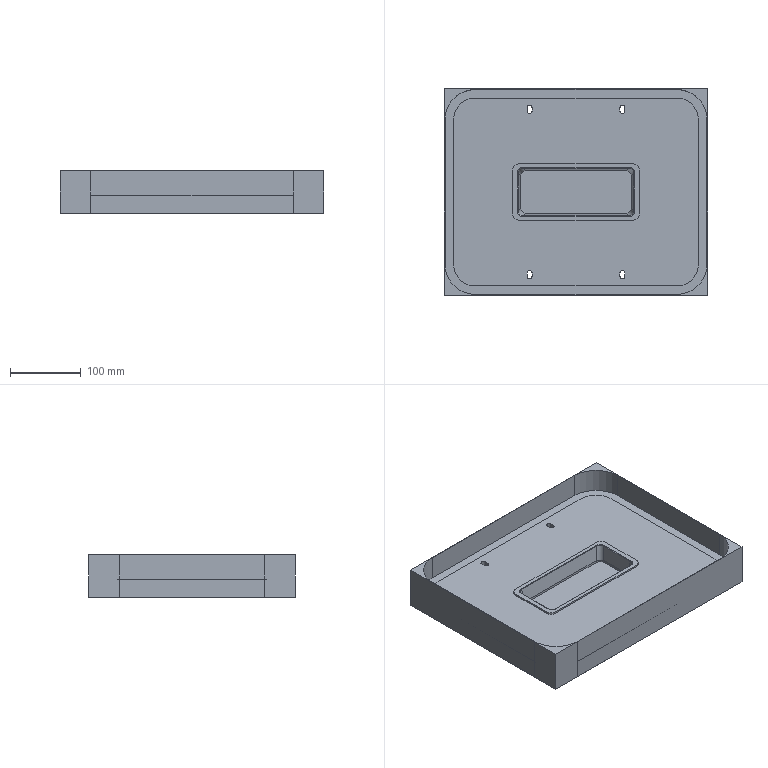NC program | NX | posted with a generic post | part box 371 x 291 x 60.5 mm
Lines 10082 to 10590 of 37416:
(FACE_MILLING , TOOL : D10)
N20162 M6
N20164 G53
N20166 G17 G0 G90 X125.485 Y-138.445 S8000 M3 M8
N20168 G43 Z120.5 H0
N20170 Z28.
N20172 G94 G1 X87.323 Y-138.446 Z26. F2000.
N20174 X-132.131 Y-138.417
N20176 X-139.591 Y-138.267
N20178 X-142.074 Y-138.176
N20180 X-144.539 Y-138.074
N20182 X-146.978 Y-137.84
N20184 X-149.417 Y-137.432
N20186 X-154.31 Y-136.321
N20188 X-159.666 Y-133.782
N20190 X-164.2 Y-131.126
N20192 X-166.631 Y-129.106
N20194 X-169.215 Y-126.515
N20196 X-170.134 Y-125.466
N20198 X-171.003 Y-124.167
N20200 X-171.388 Y-123.571
N20202 X-174.024 Y-119.195
N20204 X-176.36 Y-114.266
N20206 X-177.703 Y-109.51
N20208 X-177.879 Y-107.054
N20210 X-178.056 Y-104.576
N20212 X-178.329 Y-97.141
N20214 X-178.429 Y-87.19
N20216 X-178.411 Y92.18
N20218 X-178.394 Y94.668
N20220 X-178.214 Y104.617
N20222 X-178.147 Y107.05
N20224 X-176.316 Y114.335
N20226 X-173.784 Y119.68
N20228 X-171.125 Y124.209
N20230 X-166.637 Y129.121
N20232 X-165.443 Y130.152
N20234 X-162.7 Y132.213
N20236 X-161.736 Y132.818
N20238 X-160.781 Y133.416
N20240 X-154.243 Y136.352
N20242 X-147.014 Y138.144
N20244 X-137.114 Y138.373
N20246 X-129.641 Y138.425
N20248 X137.115
N20250 X144.541 Y138.053
N20252 X146.987 Y137.819
N20254 X149.433 Y137.424
N20256 X154.312 Y136.419
N20258 X159.614 Y133.801
N20260 X161.591 Y132.581
N20262 X163.522 Y131.344
N20264 X164.084 Y130.958
N20266 X166.649 Y129.098
N20268 X169.097 Y126.661
N20270 X170.126 Y125.477
N20272 X170.995 Y124.176
N20274 X171.392 Y123.563
N20276 X174.019 Y119.209
N20278 X176.328 Y114.251
N20280 X178.112 Y107.04
N20282 X178.27 Y104.594
N20284 X178.436 Y102.127
N20286 X178.45 Y-89.68
N20288 X178.346 Y-97.139
N20290 X178.063 Y-104.566
N20292 X177.829 Y-107.006
N20294 X177.435 Y-109.442
N20296 X176.302 Y-114.321
N20298 X174.012 Y-119.194
N20300 G2 X168.855 Y-126.469 R38.59
N20302 G1 X166.633 Y-129.122
N20304 G2 X161.765 Y-132.795 R33.332
N20306 G1 X159.726 Y-133.842
N20308 X159.243 Y-134.077
N20310 X154.275 Y-136.337
N20312 X149.421 Y-137.432
N20314 X146.984 Y-137.855
N20316 X144.548 Y-138.074
N20318 X137.113 Y-138.338
N20320 X127.155 Y-138.442
N20322 X87.323 Y-138.446
N20324 X87.324 Y-131.446
N20326 X-132.068 Y-131.417
N20328 X-139.363 Y-131.271
N20330 X-141.8 Y-131.181
N20332 X-144.059 Y-131.088
N20334 X-146.065 Y-130.896
N20336 X-148.073 Y-130.559
N20338 X-150.346 Y-130.051
N20340 X-152.017 Y-129.669
N20342 X-156.419 Y-127.573
N20344 X-160.144 Y-125.395
N20346 X-161.917 Y-123.921
N20348 X-163.95 Y-121.901
N20350 X-164.569 Y-121.196
N20352 X-166.621 Y-117.975
N20354 X-167.877 Y-115.825
N20356 X-168.891 Y-113.722
N20358 X-169.772 Y-111.841
N20360 X-170.294 Y-110.006
N20362 X-170.772 Y-108.302
N20364 X-170.897 Y-106.554
N20366 X-171.067 Y-104.172
N20368 X-171.331 Y-96.978
N20370 X-171.429 Y-87.173
N20372 X-171.411 Y92.156
N20374 X-171.394 Y94.607
N20376 X-171.217 Y104.433
N20378 X-171.171 Y106.106
N20380 X-169.708 Y111.949
N20382 X-167.573 Y116.438
N20384 X-166.597 Y118.124
N20386 X-165.481 Y120.01
N20388 X-161.748 Y124.094
N20390 X-161.046 Y124.701
N20392 X-158.734 Y126.438
N20394 X-158.018 Y126.887
N20396 X-157.41 Y127.268
N20398 X-151.995 Y129.7
N20400 X-146.072 Y131.168
N20402 X-137.024 Y131.374
N20404 X-129.625 Y131.425
N20406 X136.945
N20408 X144.026 Y131.07
N20410 X146.094 Y130.872
N20412 X148.182 Y130.535
N20414 X150.533 Y130.06
N20416 X151.989 Y129.766
N20418 X156.302 Y127.619
N20420 X160.049 Y125.238
N20422 X162.097 Y123.752
N20424 X163.98 Y121.878
N20426 X164.553 Y121.219
N20428 X166.618 Y117.981
N20430 X167.881 Y115.816
N20432 X168.853 Y113.77
N20434 X169.689 Y111.951
N20436 X171.166 Y105.982
N20438 X171.285 Y104.133
N20440 X171.436 Y101.889
N20442 X171.45 Y-89.654
N20444 X171.348 Y-96.957
N20446 X171.078 Y-104.076
N20448 X170.883 Y-106.113
N20450 X170.561 Y-108.104
N20452 X170.054 Y-110.329
N20454 X169.663 Y-112.003
N20456 X167.709 Y-116.133
N20458 X166.711 Y-117.779
N20460 X165.605 Y-119.386
N20462 X165.389 Y-119.677
N20464 X163.475 Y-121.991
N20466 X161.626 Y-124.199
N20468 X160.985 Y-124.754
N20470 X159.979 Y-125.547
N20472 X158.311 Y-126.7
N20474 X156.593 Y-127.581
N20476 X156.244 Y-127.752
N20478 X153.835 Y-128.862
N20480 X152.06 Y-129.662
N20482 X150.355 Y-130.051
N20484 X148.058 Y-130.564
N20486 X146.072 Y-130.909
N20488 X144.089 Y-131.087
N20490 X136.945 Y-131.34
N20492 X127.137 Y-131.442
N20494 X87.324 Y-131.446
N20496 X87.325 Y-124.446
N20498 X-132.006 Y-124.417
N20500 X-139.135 Y-124.275
N20502 X-141.527 Y-124.187
N20504 X-143.58 Y-124.101
N20506 X-145.152 Y-123.951
N20508 X-146.73 Y-123.687
N20510 X-148.803 Y-123.223
N20512 X-149.745 Y-123.008
N20514 X-150.769 Y-122.535
N20516 X-152.917 Y-121.512
N20518 X-154.582 Y-120.55
N20520 X-156.1 Y-119.654
N20522 X-157.204 Y-118.736
N20524 X-159.004 Y-116.925
N20526 X-161.572 Y-112.785
N20528 X-162.569 Y-110.718
N20530 X-163.193 Y-109.384
N20532 X-163.558 Y-108.103
N20534 X-163.841 Y-107.094
N20536 X-163.915 Y-106.055
N20538 X-164.078 Y-103.769
N20540 X-164.333 Y-96.814
N20542 X-164.429 Y-87.156
N20544 X-164.411 Y92.132
N20546 X-164.395 Y94.545
N20548 X-164.194 Y105.163
N20550 X-163.085 Y109.595
N20552 X-162.528 Y110.801
N20554 X-161.515 Y112.931
N20556 X-160.556 Y114.587
N20558 X-159.825 Y115.822
N20560 X-156.86 Y119.067
N20562 X-154.768 Y120.662
N20564 X-153.83 Y121.219
N20566 X-149.71 Y123.058
N20568 X-145.13 Y124.193
N20570 X-136.934 Y124.375
N20572 X-129.609 Y124.425
N20574 X136.775
N20576 X143.512 Y124.087
N20578 X145.202 Y123.926
N20580 X146.93 Y123.647
N20582 X149.736 Y123.08
N20584 X152.627 Y121.662
N20586 X156.013 Y119.518
N20588 X157.545 Y118.406
N20590 X158.979 Y116.961
N20592 X161.559 Y112.811
N20594 X162.512 Y110.805
N20596 X163.062 Y109.609
N20598 X164.219 Y104.923
N20600 X164.3 Y103.673
N20602 X164.436 Y101.651
N20604 X164.432 Y-92.024
N20606 X164.278 Y-99.133
N20608 X164.185 Y-101.518
N20610 X164.093 Y-103.587
N20612 X163.937 Y-105.219
N20614 X163.686 Y-106.765
N20616 X163.233 Y-108.755
N20618 X163.008 Y-109.717
N20620 X162.522 Y-110.771
N20622 X161.58 Y-112.739
N20624 X160.83 Y-113.977
N20626 X159.697 Y-115.576
N20628 X156.524 Y-119.357
N20630 X155.818 Y-119.913
N20632 X154.707 Y-120.681
N20634 X153.46 Y-121.321
N20636 X153.244 Y-121.427
N20638 X150.931 Y-122.492
N20640 X149.821 Y-122.993
N20642 X148.813 Y-123.223
N20644 X146.696 Y-123.696
N20646 X145.159 Y-123.963
N20648 X143.631 Y-124.1
N20650 X136.776 Y-124.342
N20652 X127.119 Y-124.442
N20654 X87.325 Y-124.446
N20656 X87.327 Y-117.446
N20658 X-131.944 Y-117.418
N20660 X-138.906 Y-117.278
N20662 X-141.253 Y-117.192
N20664 X-143.101 Y-117.115
N20666 X-144.239 Y-117.006
N20668 X-145.386 Y-116.814
N20670 X-147.472 Y-116.347
N20672 X-149.657 Y-115.312
N20674 X-152.058 Y-113.911
N20676 X-152.951 Y-113.095
N20678 X-153.521 Y-112.529
N20680 X-155.405 Y-109.457
N20682 X-156.615 Y-106.926
N20684 X-156.821 Y-106.2
N20686 X-156.909 Y-105.886
N20688 X-157.089 Y-103.366
N20690 X-157.334 Y-96.651
N20692 X-157.429 Y-87.14
N20694 X-157.411 Y92.108
N20696 X-157.395 Y94.484
N20698 X-157.217 Y104.22
N20700 X-156.462 Y107.241
N20702 X-155.315 Y109.669
N20704 X-154.17 Y111.634
N20706 X-152.062 Y113.94
N20708 X-150.684 Y114.961
N20710 X-147.425 Y116.415
N20712 X-144.188 Y117.218
N20714 X-134.455 Y117.399
N20716 X136.606 Y117.425
N20718 X142.997 Y117.105
N20720 G2 X147.51 Y116.381 R30.656
N20722 G1 X149.233 Y115.531
N20724 X152.247 Y113.602
N20726 X152.993 Y113.06
N20728 X153.505 Y112.551
N20730 X155.383 Y109.497
N20732 X156.434 Y107.268
N20734 X157.273 Y103.865
N20736 X157.436 Y101.412
N20738 X157.433 Y-91.952
N20740 X157.282 Y-98.889
N20742 X157.191 Y-101.226
N20744 X157.108 Y-103.098
N20746 X156.99 Y-104.325
N20748 X156.812 Y-105.427
N20750 X156.354 Y-107.431
N20752 X155.415 Y-109.406
N20754 X154.949 Y-110.174
N20756 X154.302 Y-111.115
N20758 X151.658 Y-114.279
N20760 X151.103 Y-114.663
N20762 X148.028 Y-116.123
N20764 X147.582 Y-116.324
N20766 X145.333 Y-116.828
N20768 X144.246 Y-117.016
N20770 X143.173 Y-117.113
N20772 X136.608 Y-117.344
N20774 X127.101 Y-117.442
N20776 X87.327 Y-117.446
N20778 X87.328 Y-110.446
N20780 X-131.882 Y-110.418
N20782 X-138.678 Y-110.282
N20784 X-140.979 Y-110.197
N20786 X-142.622 Y-110.129
N20788 X-143.326 Y-110.062
N20790 X-144.043 Y-109.942
N20792 X-145.189 Y-109.685
N20794 X-146.397 Y-109.111
N20796 X-147.521 Y-108.461
N20798 X-147.92 Y-108.225
N20800 G2 X-149.985 Y-104.578 R18.558
N20802 G1 X-150.189 Y-100.957
N20804 X-150.378 Y-94.243
N20806 X-150.429 Y-87.123
N20808 X-150.411 Y92.084
N20810 X-150.395 Y94.422
N20812 X-150.239 Y103.275
N20814 X-149.837 Y104.889
N20816 X-149.115 Y106.406
N20818 X-148.512 Y107.448
N20820 X-147.334 Y108.737
N20822 X-147.152 Y108.874
N20824 X-145.097 Y109.784
N20826 X-143.245 Y110.241
N20828 X-134.398 Y110.4
N20830 X136.436 Y110.425
N20832 X142.483 Y110.122
N20834 X143.416 Y110.033
N20836 X143.933 Y109.949
N20838 X144.427 Y109.869
N20840 X145.204 Y109.712
N20842 X145.838 Y109.399
N20844 X148.137 Y107.935
N20846 X149.207 Y106.184
N20848 X149.804 Y104.929
N20850 X150.33 Y102.752
N20852 X150.437 Y101.174
N20854 X150.433 Y-91.88
N20856 X150.287 Y-98.645
N20858 X150.197 Y-100.933
N20860 X150.123 Y-102.608
N20862 X149.937 Y-104.089
N20864 G2 X148.46 Y-107.195 R6.229
N20866 G1 X147.091 Y-108.847
N20868 X145.341 Y-109.653
N20870 X143.334 Y-110.07
N20872 X138.687 Y-110.282
N20874 X131.874 Y-110.418
N20876 X87.328 Y-110.446
N20878 X87.329 Y-103.446
N20880 X-131.82 Y-103.418
N20882 X-138.45 Y-103.285
N20884 X-142.413 Y-103.117
N20886 X-142.955 Y-102.996
N20888 X-143.072 Y-102.802
N20890 X-143.097 Y-102.749
N20892 X-143.338 Y-96.324
N20894 X-143.429 Y-87.106
N20896 X-143.411 Y92.06
N20898 X-143.395 Y94.36
N20900 X-143.26 Y102.33
N20902 X-143.214 Y102.516
N20904 X-142.941 Y103.09
N20906 X-142.861 Y103.126
N20908 X-142.303 Y103.264
N20910 X-134.342 Y103.4
N20912 X136.787
N20914 X142.524 Y103.086
N20916 X142.817 Y103.039
N20918 X143.032 Y102.87
N20920 X143.177 Y102.565
N20922 X143.383 Y101.727
N20924 X143.437 Y100.936
N20926 X143.433 Y-91.809
N20928 X143.291 Y-98.4
N20930 X143.097 Y-102.537
N20932 X143.065 Y-102.735
N20934 X142.807 Y-103.047
N20936 X142.257 Y-103.139
N20938 X134.071 Y-103.391
N20940 X117.223 Y-103.446
N20942 X87.329
N20944 X87.331 Y-96.446
N20946 X-131.757 Y-96.418
N20948 X-136.335 Y-96.343
N20950 X-136.429 Y-87.09
N20952 X-136.396 Y94.299
N20954 X-136.373 Y96.379
N20956 X-129.411 Y96.425
N20958 X136.448 Y96.408
N20960 X136.434 Y-91.737
N20962 X136.351 Y-96.343
N20964 X127.047 Y-96.442
N20966 X87.331 Y-96.446
N20968 X87.332 Y-89.446
N20970 X-129.418 Y-89.432
N20972 X-129.411 Y89.425
N20974 X129.46
N20976 X129.45 Y-89.434
N20978 X87.332 Y-89.446
N20980 X87.334 Y-82.446
N20982 X-122.429
N20984 X-122.412 Y82.425
N20986 X122.462
N20988 X122.45 Y-82.448
N20990 X87.334 Y-82.446
N20992 X87.335 Y-75.446
N20994 X-115.428 Y-75.448
N20996 X-115.413 Y75.425
N20998 X115.465
N21000 X115.451 Y-75.443
N21002 X87.335 Y-75.446
N21004 X87.336 Y-68.446
N21006 X-108.427 Y-68.448
N21008 X-108.413 Y68.425
N21010 X108.465
N21012 X108.452 Y-68.433
N21014 X87.336 Y-68.446
N21016 X87.338 Y-61.446
N21018 X-101.426 Y-61.447
N21020 X-101.414 Y61.425
N21022 X101.464
N21024 X101.462 Y36.998
N21026 X94.462 Y36.999
N21028 G3 X80.5 Y45.9 R15.4
N21030 G1 X-80.5
N21032 G3 X-94.417 Y37.095 R15.4
N21034 G1 X-94.415 Y54.425
N21036 X-84.822
N21038 Y49.925
N21040 G3 X-89.915 Y48.032 R19.9
N21042 G1 Y49.925
N21044 X-84.822
N21046 Y54.425
N21048 X84.822
N21050 Y49.925
N21052 X89.963
N21054 Y48.006
N21056 G3 X84.822 Y49.925 R19.9
N21058 G1 Y54.425
N21060 X94.463
N21062 X94.462 Y36.999
N21064 X101.462 Y36.998
N21066 X101.452 Y-61.442
N21068 X87.338 Y-61.446
N21070 X87.339 Y-54.446
N21072 X-94.426
N21074 X-94.424 Y-37.079
N21076 X-95.798 Y-32.271
N21078 G2 X-95.9 Y-30.5 R15.4
N21080 G1 Y30.5
N21082 G2 X-95.796 Y32.289 R15.4
N21084 X-96.417 Y32.512 R5.
N21086 G1 X-96.424 Y-32.496
N21088 G2 X-95.798 Y-32.271 R5.
N21090 G1 X-94.424 Y-37.079
N21092 G3 X-83.774 Y-45.548 R15.4
N21094 G1 X-84.731 Y-49.945
N21096 X-89.925 Y-49.946
N21098 Y-48.026
N21100 G3 X-84.731 Y-49.945 R19.9
N21102 G1 X-83.774 Y-45.548
N21104 G3 X-80.5 Y-45.9 R15.4
N21106 G1 X80.5
N21108 G3 X94.455 Y-37.014 R15.4
N21110 G1 X96.455 Y-32.431
N21112 X96.461 Y32.416
N21114 G2 X95.808 Y32.183 R5.
N21116 X95.9 Y30.5 R15.4
N21118 G1 Y-30.5
N21120 G2 X95.806 Y-32.2 R15.4
N21122 X96.455 Y-32.431 R5.
N21124 G1 X94.455 Y-37.014
N21126 X93.186 Y-36.421
N21128 G2 X80.5 Y-44.5 R14.
N21130 G1 X-80.5
N21132 G2 X-94.5 Y-30.5 R14.
N21134 G1 Y30.5
N21136 G2 X-80.5 Y44.5 R14.
N21138 G1 X80.5
N21140 G2 X94.5 Y30.5 R14.
N21142 G1 Y-30.5
N21144 G2 X93.186 Y-36.421 R14.
N21146 G1 X94.455 Y-37.014
N21148 X94.453 Y-54.447
N21150 X87.339 Y-54.446
N21152 X87.34 Y-49.946
N21154 X84.727
N21156 G3 X89.954 Y-48.011 R19.9
N21158 G1 X89.953 Y-49.947
N21160 X89.776
N21162 X87.34 Y-49.946
N21164 G3 X85.34 Y-51.946 R2.
N21166 G1 Z27.
N21168 G0 Z120.5
N21170 M9
N21172 M5